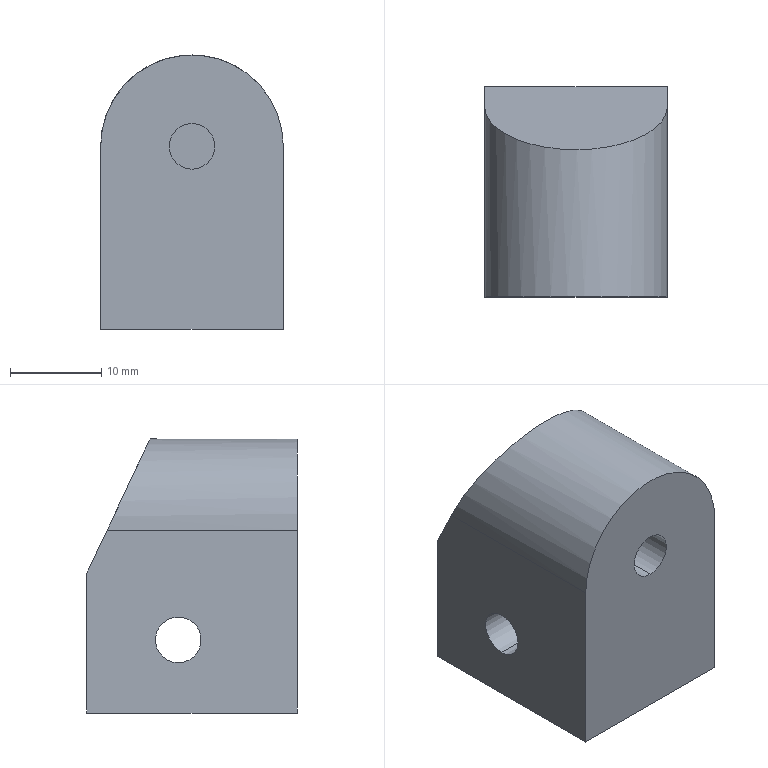Part | SolidWorks | features ICE 3, Extrusion 1 | 1 solid | 12 faces | box 20 x 23 x 30 mm | volume 11422 mm3 | plane 7 | cylinder 5 | commonest cylinder face diameters 5 x4 20 x1
STEP:
#1=CARTESIAN_POINT('',(-10.,13.,-9.5));
#2=VERTEX_POINT('',#1);
#3=CARTESIAN_POINT('',(-10.,13.,-14.5));
#4=VERTEX_POINT('',#3);
#5=CARTESIAN_POINT('',(-10.,13.,-12.));
#6=DIRECTION('',(1.,0.,0.));
#7=DIRECTION('',(0.,0.,-1.));
#8=AXIS2_PLACEMENT_3D('',#5,#6,#7);
#9=CIRCLE('',#8,2.5);
#10=EDGE_CURVE('',#2,#4,#9,.T.);
#11=ORIENTED_EDGE('',*,*,#10,.F.);
#12=CARTESIAN_POINT('',(10.,13.,-9.5));
#13=VERTEX_POINT('',#12);
#14=CARTESIAN_POINT('',(-52.,13.,-9.5));
#15=DIRECTION('',(1.,0.,0.));
#16=VECTOR('',#15,1000.);
#17=LINE('',#14,#16);
#18=EDGE_CURVE('',#2,#13,#17,.T.);
#19=ORIENTED_EDGE('',*,*,#18,.T.);
#20=CARTESIAN_POINT('',(10.,13.,-14.5));
#21=VERTEX_POINT('',#20);
#22=CARTESIAN_POINT('',(10.,13.,-12.));
#23=DIRECTION('',(1.,0.,0.));
#24=DIRECTION('',(0.,0.,-1.));
#25=AXIS2_PLACEMENT_3D('',#22,#23,#24);
#26=CIRCLE('',#25,2.5);
#27=EDGE_CURVE('',#13,#21,#26,.T.);
#28=ORIENTED_EDGE('',*,*,#27,.T.);
#29=CARTESIAN_POINT('',(-52.,13.,-14.5));
#30=DIRECTION('',(1.,0.,0.));
#31=VECTOR('',#30,1000.);
#32=LINE('',#29,#31);
#33=EDGE_CURVE('',#4,#21,#32,.T.);
#34=ORIENTED_EDGE('',*,*,#33,.F.);
#35=EDGE_LOOP('',(#11,#19,#28,#34));
#36=FACE_OUTER_BOUND('',#35,.T.);
#37=CARTESIAN_POINT('',(-52.,13.,-12.));
#38=DIRECTION('',(1.,0.,0.));
#39=DIRECTION('',(0.,0.,-1.));
#40=AXIS2_PLACEMENT_3D('',#37,#38,#39);
#41=CYLINDRICAL_SURFACE('',#40,2.5);
#42=ADVANCED_FACE('',(#36),#41,.F.);
#43=CARTESIAN_POINT('',(0.,12.,2.5));
#44=VERTEX_POINT('',#43);
#45=CARTESIAN_POINT('',(0.,12.,-2.5));
#46=VERTEX_POINT('',#45);
#47=CARTESIAN_POINT('',(0.,12.,0.));
#48=DIRECTION('',(0.,-1.,0.));
#49=DIRECTION('',(0.,0.,-1.));
#50=AXIS2_PLACEMENT_3D('',#47,#48,#49);
#51=CIRCLE('',#50,2.5);
#52=EDGE_CURVE('',#44,#46,#51,.T.);
#53=ORIENTED_EDGE('',*,*,#52,.F.);
#54=CARTESIAN_POINT('',(0.,0.,2.5));
#55=VERTEX_POINT('',#54);
#56=CARTESIAN_POINT('',(0.,12.,2.5));
#57=DIRECTION('',(0.,-1.,0.));
#58=VECTOR('',#57,1000.);
#59=LINE('',#56,#58);
#60=EDGE_CURVE('',#44,#55,#59,.T.);
#61=ORIENTED_EDGE('',*,*,#60,.T.);
#62=CARTESIAN_POINT('',(0.,0.,-2.5));
#63=VERTEX_POINT('',#62);
#64=CARTESIAN_POINT('',(0.,0.,0.));
#65=DIRECTION('',(0.,-1.,0.));
#66=DIRECTION('',(0.,0.,-1.));
#67=AXIS2_PLACEMENT_3D('',#64,#65,#66);
#68=CIRCLE('',#67,2.5);
#69=EDGE_CURVE('',#55,#63,#68,.T.);
#70=ORIENTED_EDGE('',*,*,#69,.T.);
#71=CARTESIAN_POINT('',(0.,12.,-2.5));
#72=DIRECTION('',(0.,-1.,0.));
#73=VECTOR('',#72,1000.);
#74=LINE('',#71,#73);
#75=EDGE_CURVE('',#46,#63,#74,.T.);
#76=ORIENTED_EDGE('',*,*,#75,.F.);
#77=EDGE_LOOP('',(#53,#61,#70,#76));
#78=FACE_OUTER_BOUND('',#77,.T.);
#79=CARTESIAN_POINT('',(0.,12.,0.));
#80=DIRECTION('',(0.,-1.,0.));
#81=DIRECTION('',(0.,0.,-1.));
#82=AXIS2_PLACEMENT_3D('',#79,#80,#81);
#83=CYLINDRICAL_SURFACE('',#82,2.5);
#84=ADVANCED_FACE('',(#78),#83,.F.);
#85=CARTESIAN_POINT('',(10.,20.8,0.));
#86=VERTEX_POINT('',#85);
#87=CARTESIAN_POINT('',(-10.,20.8,0.));
#88=VERTEX_POINT('',#87);
#89=CARTESIAN_POINT('',(10.,20.8,0.));
#90=CARTESIAN_POINT('',(10.,11.394,20.));
#91=CARTESIAN_POINT('',(-10.,11.394,20.));
#92=CARTESIAN_POINT('',(-10.,20.8,0.));
#93=(BOUNDED_CURVE()B_SPLINE_CURVE(3,(#89,#90,#91,#92),.UNSPECIFIED.,.F.,.T.)B_SPLINE_CURVE_WITH_KNOTS((4,4),(4.712,7.854),.UNSPECIFIED.)CURVE()GEOMETRIC_REPRESENTATION_ITEM()RATIONAL_B_SPLINE_CURVE((1.,0.3333,0.3333,1.))REPRESENTATION_ITEM(''));
#94=EDGE_CURVE('',#86,#88,#93,.T.);
#95=ORIENTED_EDGE('',*,*,#94,.T.);
#96=CARTESIAN_POINT('',(-10.,0.,0.));
#97=VERTEX_POINT('',#96);
#98=CARTESIAN_POINT('',(-10.,23.,0.));
#99=DIRECTION('',(0.,-1.,0.));
#100=VECTOR('',#99,1000.);
#101=LINE('',#98,#100);
#102=EDGE_CURVE('',#88,#97,#101,.T.);
#103=ORIENTED_EDGE('',*,*,#102,.T.);
#104=CARTESIAN_POINT('',(10.,0.,0.));
#105=VERTEX_POINT('',#104);
#106=CARTESIAN_POINT('',(0.,0.,0.));
#107=DIRECTION('',(0.,1.,0.));
#108=DIRECTION('',(0.,0.,1.));
#109=AXIS2_PLACEMENT_3D('',#106,#107,#108);
#110=CIRCLE('',#109,10.);
#111=EDGE_CURVE('',#97,#105,#110,.T.);
#112=ORIENTED_EDGE('',*,*,#111,.T.);
#113=CARTESIAN_POINT('',(10.,23.,0.));
#114=DIRECTION('',(0.,-1.,0.));
#115=VECTOR('',#114,1000.);
#116=LINE('',#113,#115);
#117=EDGE_CURVE('',#86,#105,#116,.T.);
#118=ORIENTED_EDGE('',*,*,#117,.F.);
#119=EDGE_LOOP('',(#95,#103,#112,#118));
#120=FACE_OUTER_BOUND('',#119,.T.);
#121=CARTESIAN_POINT('',(0.,23.,0.));
#122=DIRECTION('',(0.,-1.,0.));
#123=DIRECTION('',(0.,0.,-1.));
#124=AXIS2_PLACEMENT_3D('',#121,#122,#123);
#125=CYLINDRICAL_SURFACE('',#124,10.);
#126=ADVANCED_FACE('',(#120),#125,.T.);
#127=CARTESIAN_POINT('',(10.,13.,-12.));
#128=DIRECTION('',(1.,0.,0.));
#129=DIRECTION('',(0.,0.,-1.));
#130=AXIS2_PLACEMENT_3D('',#127,#128,#129);
#131=CIRCLE('',#130,2.5);
#132=EDGE_CURVE('',#21,#13,#131,.T.);
#133=ORIENTED_EDGE('',*,*,#132,.F.);
#134=ORIENTED_EDGE('',*,*,#27,.F.);
#135=EDGE_LOOP('',(#133,#134));
#136=FACE_BOUND('',#135,.T.);
#137=CARTESIAN_POINT('',(10.,23.,-4.677));
#138=VERTEX_POINT('',#137);
#139=CARTESIAN_POINT('',(10.,23.,-20.));
#140=VERTEX_POINT('',#139);
#141=CARTESIAN_POINT('',(10.,23.,-20.));
#142=DIRECTION('',(0.,0.,-1.));
#143=VECTOR('',#142,1000.);
#144=LINE('',#141,#143);
#145=EDGE_CURVE('',#138,#140,#144,.T.);
#146=ORIENTED_EDGE('',*,*,#145,.F.);
#147=CARTESIAN_POINT('',(10.,16.097,10.));
#148=DIRECTION('',(0.,0.4256,-0.9049));
#149=VECTOR('',#148,1000.);
#150=LINE('',#147,#149);
#151=EDGE_CURVE('',#86,#138,#150,.T.);
#152=ORIENTED_EDGE('',*,*,#151,.F.);
#153=ORIENTED_EDGE('',*,*,#117,.T.);
#154=CARTESIAN_POINT('',(10.,0.,-20.));
#155=VERTEX_POINT('',#154);
#156=CARTESIAN_POINT('',(10.,0.,-20.));
#157=DIRECTION('',(0.,0.,-1.));
#158=VECTOR('',#157,1000.);
#159=LINE('',#156,#158);
#160=EDGE_CURVE('',#105,#155,#159,.T.);
#161=ORIENTED_EDGE('',*,*,#160,.T.);
#162=CARTESIAN_POINT('',(10.,23.,-20.));
#163=DIRECTION('',(0.,-1.,0.));
#164=VECTOR('',#163,1000.);
#165=LINE('',#162,#164);
#166=EDGE_CURVE('',#140,#155,#165,.T.);
#167=ORIENTED_EDGE('',*,*,#166,.F.);
#168=EDGE_LOOP('',(#146,#152,#153,#161,#167));
#169=FACE_OUTER_BOUND('',#168,.T.);
#170=CARTESIAN_POINT('',(10.,23.,-20.));
#171=DIRECTION('',(-1.,0.,0.));
#172=DIRECTION('',(0.,0.,1.));
#173=AXIS2_PLACEMENT_3D('',#170,#171,#172);
#174=PLANE('',#173);
#175=ADVANCED_FACE('',(#136,#169),#174,.F.);
#176=CARTESIAN_POINT('',(-10.,0.,-20.));
#177=VERTEX_POINT('',#176);
#178=CARTESIAN_POINT('',(-10.,0.,-20.));
#179=DIRECTION('',(-1.,0.,0.));
#180=VECTOR('',#179,1000.);
#181=LINE('',#178,#180);
#182=EDGE_CURVE('',#155,#177,#181,.T.);
#183=ORIENTED_EDGE('',*,*,#182,.T.);
#184=CARTESIAN_POINT('',(-10.,23.,-20.));
#185=VERTEX_POINT('',#184);
#186=CARTESIAN_POINT('',(-10.,23.,-20.));
#187=DIRECTION('',(0.,-1.,0.));
#188=VECTOR('',#187,1000.);
#189=LINE('',#186,#188);
#190=EDGE_CURVE('',#185,#177,#189,.T.);
#191=ORIENTED_EDGE('',*,*,#190,.F.);
#192=CARTESIAN_POINT('',(-10.,23.,-20.));
#193=DIRECTION('',(-1.,0.,0.));
#194=VECTOR('',#193,1000.);
#195=LINE('',#192,#194);
#196=EDGE_CURVE('',#140,#185,#195,.T.);
#197=ORIENTED_EDGE('',*,*,#196,.F.);
#198=ORIENTED_EDGE('',*,*,#166,.T.);
#199=EDGE_LOOP('',(#183,#191,#197,#198));
#200=FACE_OUTER_BOUND('',#199,.T.);
#201=CARTESIAN_POINT('',(-10.,23.,-20.));
#202=DIRECTION('',(0.,0.,1.));
#203=DIRECTION('',(1.,0.,0.));
#204=AXIS2_PLACEMENT_3D('',#201,#202,#203);
#205=PLANE('',#204);
#206=ADVANCED_FACE('',(#200),#205,.F.);
#207=CARTESIAN_POINT('',(-10.,13.,-12.));
#208=DIRECTION('',(1.,0.,0.));
#209=DIRECTION('',(0.,0.,-1.));
#210=AXIS2_PLACEMENT_3D('',#207,#208,#209);
#211=CIRCLE('',#210,2.5);
#212=EDGE_CURVE('',#4,#2,#211,.T.);
#213=ORIENTED_EDGE('',*,*,#212,.T.);
#214=ORIENTED_EDGE('',*,*,#10,.T.);
#215=EDGE_LOOP('',(#213,#214));
#216=FACE_BOUND('',#215,.T.);
#217=ORIENTED_EDGE('',*,*,#102,.F.);
#218=CARTESIAN_POINT('',(-10.,23.,-4.677));
#219=VERTEX_POINT('',#218);
#220=CARTESIAN_POINT('',(-10.,21.199,-0.8472));
#221=DIRECTION('',(0.,0.4256,-0.9049));
#222=VECTOR('',#221,1000.);
#223=LINE('',#220,#222);
#224=EDGE_CURVE('',#88,#219,#223,.T.);
#225=ORIENTED_EDGE('',*,*,#224,.T.);
#226=CARTESIAN_POINT('',(-10.,23.,0.));
#227=DIRECTION('',(0.,0.,1.));
#228=VECTOR('',#227,1000.);
#229=LINE('',#226,#228);
#230=EDGE_CURVE('',#185,#219,#229,.T.);
#231=ORIENTED_EDGE('',*,*,#230,.F.);
#232=ORIENTED_EDGE('',*,*,#190,.T.);
#233=CARTESIAN_POINT('',(-10.,0.,0.));
#234=DIRECTION('',(0.,0.,1.));
#235=VECTOR('',#234,1000.);
#236=LINE('',#233,#235);
#237=EDGE_CURVE('',#177,#97,#236,.T.);
#238=ORIENTED_EDGE('',*,*,#237,.T.);
#239=EDGE_LOOP('',(#217,#225,#231,#232,#238));
#240=FACE_OUTER_BOUND('',#239,.T.);
#241=CARTESIAN_POINT('',(-10.,23.,0.));
#242=DIRECTION('',(1.,0.,0.));
#243=DIRECTION('',(0.,0.,-1.));
#244=AXIS2_PLACEMENT_3D('',#241,#242,#243);
#245=PLANE('',#244);
#246=ADVANCED_FACE('',(#216,#240),#245,.F.);
#247=CARTESIAN_POINT('',(0.,23.,-4.677));
#248=DIRECTION('',(-1.,0.,0.));
#249=VECTOR('',#248,1000.);
#250=LINE('',#247,#249);
#251=EDGE_CURVE('',#138,#219,#250,.T.);
#252=ORIENTED_EDGE('',*,*,#251,.F.);
#253=ORIENTED_EDGE('',*,*,#145,.T.);
#254=ORIENTED_EDGE('',*,*,#196,.T.);
#255=ORIENTED_EDGE('',*,*,#230,.T.);
#256=EDGE_LOOP('',(#252,#253,#254,#255));
#257=FACE_OUTER_BOUND('',#256,.T.);
#258=CARTESIAN_POINT('',(0.,23.,0.));
#259=DIRECTION('',(0.,1.,0.));
#260=DIRECTION('',(0.,0.,1.));
#261=AXIS2_PLACEMENT_3D('',#258,#259,#260);
#262=PLANE('',#261);
#263=ADVANCED_FACE('',(#257),#262,.T.);
#264=CARTESIAN_POINT('',(0.,0.,0.));
#265=DIRECTION('',(0.,-1.,0.));
#266=DIRECTION('',(0.,0.,-1.));
#267=AXIS2_PLACEMENT_3D('',#264,#265,#266);
#268=CIRCLE('',#267,2.5);
#269=EDGE_CURVE('',#63,#55,#268,.T.);
#270=ORIENTED_EDGE('',*,*,#269,.F.);
#271=ORIENTED_EDGE('',*,*,#69,.F.);
#272=EDGE_LOOP('',(#270,#271));
#273=FACE_BOUND('',#272,.T.);
#274=ORIENTED_EDGE('',*,*,#111,.F.);
#275=ORIENTED_EDGE('',*,*,#237,.F.);
#276=ORIENTED_EDGE('',*,*,#182,.F.);
#277=ORIENTED_EDGE('',*,*,#160,.F.);
#278=EDGE_LOOP('',(#274,#275,#276,#277));
#279=FACE_OUTER_BOUND('',#278,.T.);
#280=CARTESIAN_POINT('',(0.,0.,0.));
#281=DIRECTION('',(0.,1.,0.));
#282=DIRECTION('',(0.,0.,1.));
#283=AXIS2_PLACEMENT_3D('',#280,#281,#282);
#284=PLANE('',#283);
#285=ADVANCED_FACE('',(#273,#279),#284,.F.);
#286=ORIENTED_EDGE('',*,*,#60,.F.);
#287=CARTESIAN_POINT('',(0.,12.,0.));
#288=DIRECTION('',(0.,-1.,0.));
#289=DIRECTION('',(0.,0.,-1.));
#290=AXIS2_PLACEMENT_3D('',#287,#288,#289);
#291=CIRCLE('',#290,2.5);
#292=EDGE_CURVE('',#46,#44,#291,.T.);
#293=ORIENTED_EDGE('',*,*,#292,.F.);
#294=ORIENTED_EDGE('',*,*,#75,.T.);
#295=ORIENTED_EDGE('',*,*,#269,.T.);
#296=EDGE_LOOP('',(#286,#293,#294,#295));
#297=FACE_OUTER_BOUND('',#296,.T.);
#298=CARTESIAN_POINT('',(0.,12.,0.));
#299=DIRECTION('',(0.,-1.,0.));
#300=DIRECTION('',(0.,0.,-1.));
#301=AXIS2_PLACEMENT_3D('',#298,#299,#300);
#302=CYLINDRICAL_SURFACE('',#301,2.5);
#303=ADVANCED_FACE('',(#297),#302,.F.);
#304=ORIENTED_EDGE('',*,*,#292,.T.);
#305=ORIENTED_EDGE('',*,*,#52,.T.);
#306=EDGE_LOOP('',(#304,#305));
#307=FACE_OUTER_BOUND('',#306,.T.);
#308=CARTESIAN_POINT('',(0.,12.,0.));
#309=DIRECTION('',(0.,-1.,0.));
#310=DIRECTION('',(0.,0.,-1.));
#311=AXIS2_PLACEMENT_3D('',#308,#309,#310);
#312=PLANE('',#311);
#313=ADVANCED_FACE('',(#307),#312,.T.);
#314=ORIENTED_EDGE('',*,*,#18,.F.);
#315=ORIENTED_EDGE('',*,*,#212,.F.);
#316=ORIENTED_EDGE('',*,*,#33,.T.);
#317=ORIENTED_EDGE('',*,*,#132,.T.);
#318=EDGE_LOOP('',(#314,#315,#316,#317));
#319=FACE_OUTER_BOUND('',#318,.T.);
#320=CARTESIAN_POINT('',(-52.,13.,-12.));
#321=DIRECTION('',(1.,0.,0.));
#322=DIRECTION('',(0.,0.,-1.));
#323=AXIS2_PLACEMENT_3D('',#320,#321,#322);
#324=CYLINDRICAL_SURFACE('',#323,2.5);
#325=ADVANCED_FACE('',(#319),#324,.F.);
#326=ORIENTED_EDGE('',*,*,#151,.T.);
#327=ORIENTED_EDGE('',*,*,#251,.T.);
#328=ORIENTED_EDGE('',*,*,#224,.F.);
#329=ORIENTED_EDGE('',*,*,#94,.F.);
#330=EDGE_LOOP('',(#326,#327,#328,#329));
#331=FACE_OUTER_BOUND('',#330,.T.);
#332=CARTESIAN_POINT('',(-16.,16.097,10.));
#333=DIRECTION('',(0.,-0.9049,-0.4256));
#334=DIRECTION('',(0.,0.4256,-0.9049));
#335=AXIS2_PLACEMENT_3D('',#332,#333,#334);
#336=PLANE('',#335);
#337=ADVANCED_FACE('',(#331),#336,.F.);
#338=CLOSED_SHELL('',(#42,#84,#126,#175,#206,#246,#263,#285,#303,#313,#325,#337));
#339=MANIFOLD_SOLID_BREP('',#338);
#340=CARTESIAN_POINT('',(0.,0.,0.));
#341=DIRECTION('',(0.,0.,1.));
#342=DIRECTION('',(1.,0.,0.));
#343=AXIS2_PLACEMENT_3D('',#340,#341,#342);
#344=(LENGTH_UNIT()NAMED_UNIT(*)SI_UNIT(.MILLI.,.METRE.));
#345=UNCERTAINTY_MEASURE_WITH_UNIT(LENGTH_MEASURE(0.00001),#344,'','');
#346=(NAMED_UNIT(*)PLANE_ANGLE_UNIT()SI_UNIT($,.RADIAN.));
#347=(NAMED_UNIT(*)SI_UNIT($,.STERADIAN.)SOLID_ANGLE_UNIT());
#348=(GEOMETRIC_REPRESENTATION_CONTEXT(3)GLOBAL_UNCERTAINTY_ASSIGNED_CONTEXT((#345))GLOBAL_UNIT_ASSIGNED_CONTEXT((#344,#346,#347))REPRESENTATION_CONTEXT('',''));
#349=ADVANCED_BREP_SHAPE_REPRESENTATION('',(#339,#343),#348);